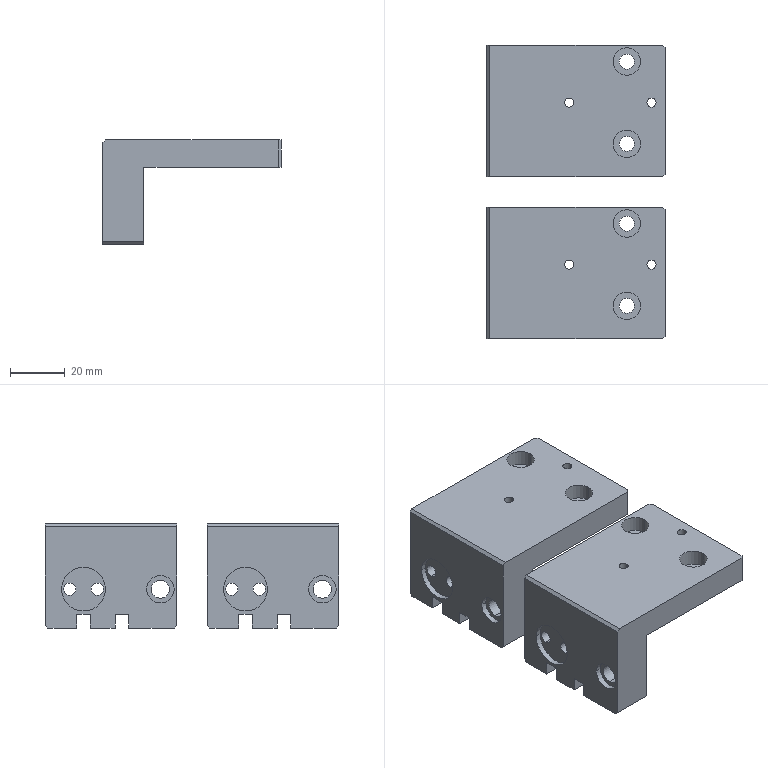Part | 2 solids | 128 faces | box 65 x 107 x 38 mm | volume 93964 mm3 | cylinder 64 | plane 56 | cone 8 | commonest cylinder face diameters 10 x12 3.3 x8 4 x8 4.5 x8 5.5 x8 8 x8